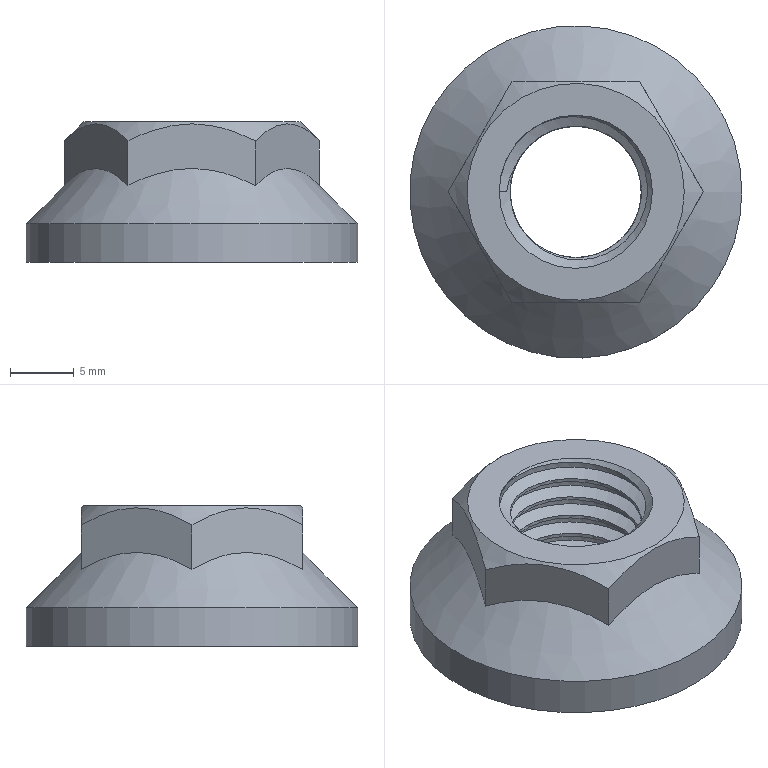Part | NX | features CYLINDER 2, DATUM_CSYS 2, CHAMFER 1, CONE 1, DELETE FACE 1, EXTRUDE 1, HOLE PACKAGE 1, INTERSECT 1, SIMPLE HOLE 1, SKETCH 1, SYMBOLIC_THREAD 1, THREADS 1 | 1 solid | 19 faces | box 26 x 26 x 11 mm | volume 3067 mm3 | plane 10 | cone 4 | cylinder 3 | spline 2 | commonest cylinder face diameters 10.3 x1 12 x1 26 x1
STEP:
#1=CARTESIAN_POINT('',(-4.994,-8.65,9.5));
#2=VERTEX_POINT('',#1);
#3=CARTESIAN_POINT('',(-4.994,-8.65,6.012));
#4=VERTEX_POINT('',#3);
#5=CARTESIAN_POINT('',(-4.994,-8.65,11.));
#6=DIRECTION('',(0.,0.,-1.));
#7=VECTOR('',#6,1000.);
#8=LINE('',#5,#7);
#9=EDGE_CURVE('',#2,#4,#8,.T.);
#10=ORIENTED_EDGE('',*,*,#9,.T.);
#11=CARTESIAN_POINT('',(4.994,-8.65,6.012));
#12=VERTEX_POINT('',#11);
#13=CARTESIAN_POINT('',(-4.994,-8.65,6.012));
#14=CARTESIAN_POINT('',(-3.437,-8.65,6.79));
#15=CARTESIAN_POINT('',(0.004869,-8.65,7.912));
#16=CARTESIAN_POINT('',(3.447,-8.65,6.785));
#17=CARTESIAN_POINT('',(4.994,-8.65,6.012));
#18=B_SPLINE_CURVE_WITH_KNOTS('',3,(#13,#14,#15,#16,#17),.UNSPECIFIED.,.F.,.F.,(4,1,4),(0.008324,0.01351,0.01869),.UNSPECIFIED.);
#19=EDGE_CURVE('',#4,#12,#18,.T.);
#20=ORIENTED_EDGE('',*,*,#19,.T.);
#21=CARTESIAN_POINT('',(4.994,-8.65,9.5));
#22=VERTEX_POINT('',#21);
#23=CARTESIAN_POINT('',(4.994,-8.65,11.));
#24=DIRECTION('',(0.,0.,-1.));
#25=VECTOR('',#24,1000.);
#26=LINE('',#23,#25);
#27=EDGE_CURVE('',#22,#12,#26,.T.);
#28=ORIENTED_EDGE('',*,*,#27,.F.);
#29=CARTESIAN_POINT('',(-4.994,-8.65,9.5));
#30=CARTESIAN_POINT('',(-3.445,-8.65,10.275));
#31=CARTESIAN_POINT('',(0.002531,-8.65,11.403));
#32=CARTESIAN_POINT('',(3.449,-8.65,10.273));
#33=CARTESIAN_POINT('',(4.994,-8.65,9.5));
#34=B_SPLINE_CURVE_WITH_KNOTS('',3,(#29,#30,#31,#32,#33),.UNSPECIFIED.,.F.,.F.,(4,1,4),(0.006405,0.01158,0.01676),.UNSPECIFIED.);
#35=EDGE_CURVE('',#22,#2,#34,.F.);
#36=ORIENTED_EDGE('',*,*,#35,.T.);
#37=EDGE_LOOP('',(#10,#20,#28,#36));
#38=FACE_BOUND('',#37,.T.);
#39=CARTESIAN_POINT('',(-4.994,-8.65,11.));
#40=DIRECTION('',(0.,1.,0.));
#41=DIRECTION('',(-1.,0.,0.));
#42=AXIS2_PLACEMENT_3D('',#39,#40,#41);
#43=PLANE('',#42);
#44=ADVANCED_FACE('',(#38),#43,.F.);
#45=ORIENTED_EDGE('',*,*,#27,.T.);
#46=CARTESIAN_POINT('',(9.988,0.,6.012));
#47=VERTEX_POINT('',#46);
#48=CARTESIAN_POINT('',(4.994,-8.65,6.012));
#49=CARTESIAN_POINT('',(5.384,-7.974,6.402));
#50=CARTESIAN_POINT('',(6.177,-6.602,7.066));
#51=CARTESIAN_POINT('',(7.921,-3.581,7.631));
#52=CARTESIAN_POINT('',(9.203,-1.36,6.797));
#53=CARTESIAN_POINT('',(9.988,0.,6.012));
#54=B_SPLINE_CURVE_WITH_KNOTS('',3,(#48,#49,#50,#51,#52,#53),.UNSPECIFIED.,.F.,.F.,(4,1,1,4),(0.000000254,0.00258,0.005159,0.01032),.UNSPECIFIED.);
#55=EDGE_CURVE('',#12,#47,#54,.T.);
#56=ORIENTED_EDGE('',*,*,#55,.T.);
#57=CARTESIAN_POINT('',(9.988,0.,9.5));
#58=VERTEX_POINT('',#57);
#59=CARTESIAN_POINT('',(9.988,0.,11.));
#60=DIRECTION('',(0.,0.,-1.));
#61=VECTOR('',#60,1000.);
#62=LINE('',#59,#61);
#63=EDGE_CURVE('',#58,#47,#62,.T.);
#64=ORIENTED_EDGE('',*,*,#63,.F.);
#65=CARTESIAN_POINT('',(9.988,0.,9.5));
#66=CARTESIAN_POINT('',(9.598,-0.6758,9.89));
#67=CARTESIAN_POINT('',(8.806,-2.048,10.554));
#68=CARTESIAN_POINT('',(7.061,-5.069,11.119));
#69=CARTESIAN_POINT('',(5.779,-7.29,10.285));
#70=CARTESIAN_POINT('',(4.994,-8.65,9.5));
#71=B_SPLINE_CURVE_WITH_KNOTS('',3,(#65,#66,#67,#68,#69,#70),.UNSPECIFIED.,.F.,.F.,(4,1,1,4),(0.000000254,0.00258,0.005159,0.01032),.UNSPECIFIED.);
#72=EDGE_CURVE('',#58,#22,#71,.T.);
#73=ORIENTED_EDGE('',*,*,#72,.T.);
#74=EDGE_LOOP('',(#45,#56,#64,#73));
#75=FACE_BOUND('',#74,.T.);
#76=CARTESIAN_POINT('',(4.994,-8.65,11.));
#77=DIRECTION('',(-0.866,0.5,0.));
#78=DIRECTION('',(-0.5,-0.866,0.));
#79=AXIS2_PLACEMENT_3D('',#76,#77,#78);
#80=PLANE('',#79);
#81=ADVANCED_FACE('',(#75),#80,.F.);
#82=ORIENTED_EDGE('',*,*,#63,.T.);
#83=CARTESIAN_POINT('',(4.994,8.65,6.012));
#84=VERTEX_POINT('',#83);
#85=CARTESIAN_POINT('',(9.988,0.,6.012));
#86=CARTESIAN_POINT('',(9.598,0.6758,6.402));
#87=CARTESIAN_POINT('',(8.806,2.048,7.066));
#88=CARTESIAN_POINT('',(7.061,5.069,7.631));
#89=CARTESIAN_POINT('',(5.779,7.29,6.797));
#90=CARTESIAN_POINT('',(4.994,8.65,6.012));
#91=B_SPLINE_CURVE_WITH_KNOTS('',3,(#85,#86,#87,#88,#89,#90),.UNSPECIFIED.,.F.,.F.,(4,1,1,4),(0.000000254,0.00258,0.005159,0.01032),.UNSPECIFIED.);
#92=EDGE_CURVE('',#47,#84,#91,.T.);
#93=ORIENTED_EDGE('',*,*,#92,.T.);
#94=CARTESIAN_POINT('',(4.994,8.65,9.5));
#95=VERTEX_POINT('',#94);
#96=CARTESIAN_POINT('',(4.994,8.65,11.));
#97=DIRECTION('',(0.,0.,-1.));
#98=VECTOR('',#97,1000.);
#99=LINE('',#96,#98);
#100=EDGE_CURVE('',#95,#84,#99,.T.);
#101=ORIENTED_EDGE('',*,*,#100,.F.);
#102=CARTESIAN_POINT('',(4.994,8.65,9.5));
#103=CARTESIAN_POINT('',(5.384,7.974,9.89));
#104=CARTESIAN_POINT('',(6.177,6.602,10.554));
#105=CARTESIAN_POINT('',(7.921,3.581,11.119));
#106=CARTESIAN_POINT('',(9.203,1.36,10.285));
#107=CARTESIAN_POINT('',(9.988,0.,9.5));
#108=B_SPLINE_CURVE_WITH_KNOTS('',3,(#102,#103,#104,#105,#106,#107),.UNSPECIFIED.,.F.,.F.,(4,1,1,4),(0.000000254,0.00258,0.005159,0.01032),.UNSPECIFIED.);
#109=EDGE_CURVE('',#95,#58,#108,.T.);
#110=ORIENTED_EDGE('',*,*,#109,.T.);
#111=EDGE_LOOP('',(#82,#93,#101,#110));
#112=FACE_BOUND('',#111,.T.);
#113=CARTESIAN_POINT('',(9.988,0.,11.));
#114=DIRECTION('',(-0.866,-0.5,0.));
#115=DIRECTION('',(0.5,-0.866,0.));
#116=AXIS2_PLACEMENT_3D('',#113,#114,#115);
#117=PLANE('',#116);
#118=ADVANCED_FACE('',(#112),#117,.F.);
#119=ORIENTED_EDGE('',*,*,#100,.T.);
#120=CARTESIAN_POINT('',(-4.994,8.65,6.012));
#121=VERTEX_POINT('',#120);
#122=CARTESIAN_POINT('',(-4.994,8.65,6.012));
#123=CARTESIAN_POINT('',(-3.437,8.65,6.79));
#124=CARTESIAN_POINT('',(0.004869,8.65,7.912));
#125=CARTESIAN_POINT('',(3.447,8.65,6.785));
#126=CARTESIAN_POINT('',(4.994,8.65,6.012));
#127=B_SPLINE_CURVE_WITH_KNOTS('',3,(#122,#123,#124,#125,#126),.UNSPECIFIED.,.F.,.F.,(4,1,4),(0.008324,0.01351,0.01869),.UNSPECIFIED.);
#128=EDGE_CURVE('',#84,#121,#127,.F.);
#129=ORIENTED_EDGE('',*,*,#128,.T.);
#130=CARTESIAN_POINT('',(-4.994,8.65,9.5));
#131=VERTEX_POINT('',#130);
#132=CARTESIAN_POINT('',(-4.994,8.65,11.));
#133=DIRECTION('',(0.,0.,-1.));
#134=VECTOR('',#133,1000.);
#135=LINE('',#132,#134);
#136=EDGE_CURVE('',#131,#121,#135,.T.);
#137=ORIENTED_EDGE('',*,*,#136,.F.);
#138=CARTESIAN_POINT('',(-4.994,8.65,9.5));
#139=CARTESIAN_POINT('',(-3.445,8.65,10.275));
#140=CARTESIAN_POINT('',(0.002531,8.65,11.403));
#141=CARTESIAN_POINT('',(3.449,8.65,10.273));
#142=CARTESIAN_POINT('',(4.994,8.65,9.5));
#143=B_SPLINE_CURVE_WITH_KNOTS('',3,(#138,#139,#140,#141,#142),.UNSPECIFIED.,.F.,.F.,(4,1,4),(0.006405,0.01158,0.01676),.UNSPECIFIED.);
#144=EDGE_CURVE('',#131,#95,#143,.T.);
#145=ORIENTED_EDGE('',*,*,#144,.T.);
#146=EDGE_LOOP('',(#119,#129,#137,#145));
#147=FACE_BOUND('',#146,.T.);
#148=CARTESIAN_POINT('',(4.994,8.65,11.));
#149=DIRECTION('',(0.,-1.,0.));
#150=DIRECTION('',(1.,0.,0.));
#151=AXIS2_PLACEMENT_3D('',#148,#149,#150);
#152=PLANE('',#151);
#153=ADVANCED_FACE('',(#147),#152,.F.);
#154=ORIENTED_EDGE('',*,*,#136,.T.);
#155=CARTESIAN_POINT('',(-9.988,0.,6.012));
#156=VERTEX_POINT('',#155);
#157=CARTESIAN_POINT('',(-4.994,8.65,6.012));
#158=CARTESIAN_POINT('',(-5.384,7.974,6.402));
#159=CARTESIAN_POINT('',(-6.177,6.602,7.066));
#160=CARTESIAN_POINT('',(-7.921,3.581,7.631));
#161=CARTESIAN_POINT('',(-9.203,1.36,6.797));
#162=CARTESIAN_POINT('',(-9.988,0.,6.012));
#163=B_SPLINE_CURVE_WITH_KNOTS('',3,(#157,#158,#159,#160,#161,#162),.UNSPECIFIED.,.F.,.F.,(4,1,1,4),(0.000000254,0.00258,0.005159,0.01032),.UNSPECIFIED.);
#164=EDGE_CURVE('',#121,#156,#163,.T.);
#165=ORIENTED_EDGE('',*,*,#164,.T.);
#166=CARTESIAN_POINT('',(-9.988,0.,9.5));
#167=VERTEX_POINT('',#166);
#168=CARTESIAN_POINT('',(-9.988,0.,11.));
#169=DIRECTION('',(0.,0.,-1.));
#170=VECTOR('',#169,1000.);
#171=LINE('',#168,#170);
#172=EDGE_CURVE('',#167,#156,#171,.T.);
#173=ORIENTED_EDGE('',*,*,#172,.F.);
#174=CARTESIAN_POINT('',(-9.988,0.,9.5));
#175=CARTESIAN_POINT('',(-9.598,0.6758,9.89));
#176=CARTESIAN_POINT('',(-8.806,2.048,10.554));
#177=CARTESIAN_POINT('',(-7.061,5.069,11.119));
#178=CARTESIAN_POINT('',(-5.779,7.29,10.285));
#179=CARTESIAN_POINT('',(-4.994,8.65,9.5));
#180=B_SPLINE_CURVE_WITH_KNOTS('',3,(#174,#175,#176,#177,#178,#179),.UNSPECIFIED.,.F.,.F.,(4,1,1,4),(0.000000254,0.00258,0.005159,0.01032),.UNSPECIFIED.);
#181=EDGE_CURVE('',#167,#131,#180,.T.);
#182=ORIENTED_EDGE('',*,*,#181,.T.);
#183=EDGE_LOOP('',(#154,#165,#173,#182));
#184=FACE_BOUND('',#183,.T.);
#185=CARTESIAN_POINT('',(-4.994,8.65,11.));
#186=DIRECTION('',(0.866,-0.5,0.));
#187=DIRECTION('',(0.5,0.866,0.));
#188=AXIS2_PLACEMENT_3D('',#185,#186,#187);
#189=PLANE('',#188);
#190=ADVANCED_FACE('',(#184),#189,.F.);
#191=ORIENTED_EDGE('',*,*,#172,.T.);
#192=CARTESIAN_POINT('',(-9.988,0.,6.012));
#193=CARTESIAN_POINT('',(-9.598,-0.6758,6.402));
#194=CARTESIAN_POINT('',(-8.806,-2.048,7.066));
#195=CARTESIAN_POINT('',(-7.061,-5.069,7.631));
#196=CARTESIAN_POINT('',(-5.779,-7.29,6.797));
#197=CARTESIAN_POINT('',(-4.994,-8.65,6.012));
#198=B_SPLINE_CURVE_WITH_KNOTS('',3,(#192,#193,#194,#195,#196,#197),.UNSPECIFIED.,.F.,.F.,(4,1,1,4),(0.000000254,0.00258,0.005159,0.01032),.UNSPECIFIED.);
#199=EDGE_CURVE('',#156,#4,#198,.T.);
#200=ORIENTED_EDGE('',*,*,#199,.T.);
#201=ORIENTED_EDGE('',*,*,#9,.F.);
#202=CARTESIAN_POINT('',(-4.994,-8.65,9.5));
#203=CARTESIAN_POINT('',(-5.384,-7.974,9.89));
#204=CARTESIAN_POINT('',(-6.177,-6.602,10.554));
#205=CARTESIAN_POINT('',(-7.921,-3.581,11.119));
#206=CARTESIAN_POINT('',(-9.203,-1.36,10.285));
#207=CARTESIAN_POINT('',(-9.988,0.,9.5));
#208=B_SPLINE_CURVE_WITH_KNOTS('',3,(#202,#203,#204,#205,#206,#207),.UNSPECIFIED.,.F.,.F.,(4,1,1,4),(0.000000254,0.00258,0.005159,0.01032),.UNSPECIFIED.);
#209=EDGE_CURVE('',#2,#167,#208,.T.);
#210=ORIENTED_EDGE('',*,*,#209,.T.);
#211=EDGE_LOOP('',(#191,#200,#201,#210));
#212=FACE_BOUND('',#211,.T.);
#213=CARTESIAN_POINT('',(-9.988,0.,11.));
#214=DIRECTION('',(0.866,0.5,0.));
#215=DIRECTION('',(-0.5,0.866,0.));
#216=AXIS2_PLACEMENT_3D('',#213,#214,#215);
#217=PLANE('',#216);
#218=ADVANCED_FACE('',(#212),#217,.F.);
#219=CARTESIAN_POINT('',(-6.,0.,11.));
#220=VERTEX_POINT('',#219);
#221=CARTESIAN_POINT('',(-3.737,4.694,11.));
#222=VERTEX_POINT('',#221);
#223=CARTESIAN_POINT('',(0.,0.,11.));
#224=DIRECTION('',(0.,0.,1.));
#225=DIRECTION('',(1.,0.,0.));
#226=AXIS2_PLACEMENT_3D('',#223,#224,#225);
#227=CIRCLE('',#226,6.);
#228=EDGE_CURVE('',#220,#222,#227,.F.);
#229=ORIENTED_EDGE('',*,*,#228,.T.);
#230=CARTESIAN_POINT('',(0.,0.,11.));
#231=DIRECTION('',(0.,0.,1.));
#232=DIRECTION('',(1.,0.,0.));
#233=AXIS2_PLACEMENT_3D('',#230,#231,#232);
#234=CIRCLE('',#233,6.);
#235=EDGE_CURVE('',#222,#220,#234,.F.);
#236=ORIENTED_EDGE('',*,*,#235,.T.);
#237=EDGE_LOOP('',(#229,#236));
#238=FACE_BOUND('',#237,.T.);
#239=CARTESIAN_POINT('',(8.488,0.,11.));
#240=VERTEX_POINT('',#239);
#241=CARTESIAN_POINT('',(0.,0.,11.));
#242=DIRECTION('',(0.,0.,1.));
#243=DIRECTION('',(1.,0.,0.));
#244=AXIS2_PLACEMENT_3D('',#241,#242,#243);
#245=CIRCLE('',#244,8.488);
#246=EDGE_CURVE('',#240,#240,#245,.T.);
#247=ORIENTED_EDGE('',*,*,#246,.T.);
#248=EDGE_LOOP('',(#247));
#249=FACE_BOUND('',#248,.T.);
#250=CARTESIAN_POINT('',(0.,0.,11.));
#251=DIRECTION('',(0.,0.,1.));
#252=DIRECTION('',(1.,0.,0.));
#253=AXIS2_PLACEMENT_3D('',#250,#251,#252);
#254=PLANE('',#253);
#255=ADVANCED_FACE('',(#238,#249),#254,.T.);
#256=ORIENTED_EDGE('',*,*,#246,.F.);
#257=EDGE_LOOP('',(#256));
#258=FACE_BOUND('',#257,.T.);
#259=ORIENTED_EDGE('',*,*,#35,.F.);
#260=ORIENTED_EDGE('',*,*,#72,.F.);
#261=ORIENTED_EDGE('',*,*,#109,.F.);
#262=ORIENTED_EDGE('',*,*,#144,.F.);
#263=ORIENTED_EDGE('',*,*,#181,.F.);
#264=ORIENTED_EDGE('',*,*,#209,.F.);
#265=EDGE_LOOP('',(#259,#260,#261,#262,#263,#264));
#266=FACE_BOUND('',#265,.T.);
#267=CARTESIAN_POINT('',(0.,0.,9.5));
#268=DIRECTION('',(0.,0.,-1.));
#269=DIRECTION('',(-1.,0.,0.));
#270=AXIS2_PLACEMENT_3D('',#267,#268,#269);
#271=CONICAL_SURFACE('',#270,9.988,0.7854);
#272=ADVANCED_FACE('',(#258,#266),#271,.T.);
#273=CARTESIAN_POINT('',(13.,0.,3.));
#274=VERTEX_POINT('',#273);
#275=CARTESIAN_POINT('',(0.,0.,3.));
#276=DIRECTION('',(0.,0.,1.));
#277=DIRECTION('',(1.,0.,0.));
#278=AXIS2_PLACEMENT_3D('',#275,#276,#277);
#279=CIRCLE('',#278,13.);
#280=EDGE_CURVE('',#274,#274,#279,.T.);
#281=ORIENTED_EDGE('',*,*,#280,.T.);
#282=EDGE_LOOP('',(#281));
#283=FACE_BOUND('',#282,.T.);
#284=ORIENTED_EDGE('',*,*,#19,.F.);
#285=ORIENTED_EDGE('',*,*,#199,.F.);
#286=ORIENTED_EDGE('',*,*,#164,.F.);
#287=ORIENTED_EDGE('',*,*,#128,.F.);
#288=ORIENTED_EDGE('',*,*,#92,.F.);
#289=ORIENTED_EDGE('',*,*,#55,.F.);
#290=EDGE_LOOP('',(#284,#285,#286,#287,#288,#289));
#291=FACE_BOUND('',#290,.T.);
#292=CARTESIAN_POINT('',(0.,0.,16.));
#293=DIRECTION('',(0.,0.,-1.));
#294=DIRECTION('',(1.,0.,0.));
#295=AXIS2_PLACEMENT_3D('',#292,#293,#294);
#296=CONICAL_SURFACE('',#295,0.,0.7854);
#297=ADVANCED_FACE('',(#283,#291),#296,.T.);
#298=CARTESIAN_POINT('',(-6.,0.,0.));
#299=VERTEX_POINT('',#298);
#300=CARTESIAN_POINT('',(0.,0.,0.));
#301=DIRECTION('',(0.,0.,-1.));
#302=DIRECTION('',(-1.,0.,0.));
#303=AXIS2_PLACEMENT_3D('',#300,#301,#302);
#304=CIRCLE('',#303,6.);
#305=EDGE_CURVE('',#299,#299,#304,.F.);
#306=ORIENTED_EDGE('',*,*,#305,.T.);
#307=EDGE_LOOP('',(#306));
#308=FACE_BOUND('',#307,.T.);
#309=CARTESIAN_POINT('',(13.,0.,0.));
#310=VERTEX_POINT('',#309);
#311=CARTESIAN_POINT('',(0.,0.,0.));
#312=DIRECTION('',(0.,0.,1.));
#313=DIRECTION('',(1.,0.,0.));
#314=AXIS2_PLACEMENT_3D('',#311,#312,#313);
#315=CIRCLE('',#314,13.);
#316=EDGE_CURVE('',#310,#310,#315,.T.);
#317=ORIENTED_EDGE('',*,*,#316,.F.);
#318=EDGE_LOOP('',(#317));
#319=FACE_BOUND('',#318,.T.);
#320=CARTESIAN_POINT('',(0.,0.,0.));
#321=DIRECTION('',(0.,0.,-1.));
#322=DIRECTION('',(-1.,0.,0.));
#323=AXIS2_PLACEMENT_3D('',#320,#321,#322);
#324=PLANE('',#323);
#325=ADVANCED_FACE('',(#308,#319),#324,.T.);
#326=ORIENTED_EDGE('',*,*,#280,.F.);
#327=EDGE_LOOP('',(#326));
#328=FACE_BOUND('',#327,.T.);
#329=ORIENTED_EDGE('',*,*,#316,.T.);
#330=EDGE_LOOP('',(#329));
#331=FACE_BOUND('',#330,.T.);
#332=CARTESIAN_POINT('',(0.,0.,0.));
#333=DIRECTION('',(0.,0.,1.));
#334=DIRECTION('',(1.,0.,0.));
#335=AXIS2_PLACEMENT_3D('',#332,#333,#334);
#336=CYLINDRICAL_SURFACE('',#335,13.);
#337=ADVANCED_FACE('',(#328,#331),#336,.T.);
#338=CARTESIAN_POINT('',(-4.333,-2.784,10.15));
#339=VERTEX_POINT('',#338);
#340=CARTESIAN_POINT('',(4.339,2.774,2.274));
#341=VERTEX_POINT('',#340);
#342=CARTESIAN_POINT('',(-4.333,-2.784,10.15));
#343=CARTESIAN_POINT('',(-5.161,-1.496,10.067));
#344=CARTESIAN_POINT('',(-5.577,1.793,9.904));
#345=CARTESIAN_POINT('',(-2.144,5.461,9.658));
#346=CARTESIAN_POINT('',(2.855,5.122,9.412));
#347=CARTESIAN_POINT('',(5.773,1.04,9.166));
#348=CARTESIAN_POINT('',(4.463,-3.803,8.919));
#349=CARTESIAN_POINT('',(-0.1032,-5.864,8.674));
#350=CARTESIAN_POINT('',(-4.603,-3.635,8.427));
#351=CARTESIAN_POINT('',(-5.73,1.246,8.181));
#352=CARTESIAN_POINT('',(-2.671,5.223,7.935));
#353=CARTESIAN_POINT('',(2.346,5.375,7.689));
#354=CARTESIAN_POINT('',(5.641,1.603,7.443));
#355=CARTESIAN_POINT('',(4.815,-3.349,7.197));
#356=CARTESIAN_POINT('',(0.4676,-5.845,6.951));
#357=CARTESIAN_POINT('',(-4.222,-4.072,6.705));
#358=CARTESIAN_POINT('',(-5.824,0.6857,6.458));
#359=CARTESIAN_POINT('',(-3.17,4.933,6.213));
#360=CARTESIAN_POINT('',(1.807,5.581,5.966));
#361=CARTESIAN_POINT('',(5.459,2.141,5.72));
#362=CARTESIAN_POINT('',(5.122,-2.858,5.474));
#363=CARTESIAN_POINT('',(1.034,-5.773,5.228));
#364=CARTESIAN_POINT('',(-3.802,-4.464,4.982));
#365=CARTESIAN_POINT('',(-5.865,0.1088,4.736));
#366=CARTESIAN_POINT('',(-3.632,4.604,4.489));
#367=CARTESIAN_POINT('',(1.248,5.73,4.244));
#368=CARTESIAN_POINT('',(5.225,2.666,3.997));
#369=CARTESIAN_POINT('',(5.374,-2.345,3.752));
#370=CARTESIAN_POINT('',(1.599,-5.644,3.505));
#371=CARTESIAN_POINT('',(-3.352,-4.812,3.259));
#372=CARTESIAN_POINT('',(-5.845,-0.4681,3.013));
#373=CARTESIAN_POINT('',(-4.069,4.228,2.767));
#374=CARTESIAN_POINT('',(0.6899,5.818,2.521));
#375=CARTESIAN_POINT('',(3.514,4.065,2.357));
#376=CARTESIAN_POINT('',(4.339,2.774,2.274));
#377=B_SPLINE_CURVE_WITH_KNOTS('',3,(#342,#343,#344,#345,#346,#347,#348,#349,#350,#351,#352,#353,#354,#355,#356,#357,#358,#359,#360,#361,#362,#363,#364,#365,#366,#367,#368,#369,#370,#371,#372,#373,#374,#375,#376),.UNSPECIFIED.,.F.,.F.,(4,1,1,1,1,1,1,1,1,1,1,1,1,1,1,1,1,1,1,1,1,1,1,1,1,1,1,1,1,1,1,1,4),(0.,0.004536,0.009071,0.01361,0.01814,0.02268,0.02721,0.03175,0.03629,0.04082,0.04536,0.04989,0.05443,0.05896,0.0635,0.06803,0.07257,0.07711,0.08164,0.08618,0.09071,0.09525,0.09978,0.1043,0.1089,0.1134,0.1179,0.1225,0.127,0.1315,0.1361,0.1406,0.1451),.UNSPECIFIED.);
#378=EDGE_CURVE('',#339,#341,#377,.T.);
#379=ORIENTED_EDGE('',*,*,#378,.T.);
#380=CARTESIAN_POINT('',(4.339,2.774,0.85));
#381=VERTEX_POINT('',#380);
#382=CARTESIAN_POINT('',(4.339,2.774,11.));
#383=DIRECTION('',(0.,0.,-1.));
#384=VECTOR('',#383,1000.);
#385=LINE('',#382,#384);
#386=EDGE_CURVE('',#341,#381,#385,.T.);
#387=ORIENTED_EDGE('',*,*,#386,.T.);
#388=CARTESIAN_POINT('',(3.676,3.607,0.85));
#389=VERTEX_POINT('',#388);
#390=CARTESIAN_POINT('',(0.,0.,0.85));
#391=DIRECTION('',(0.,0.,-1.));
#392=DIRECTION('',(-1.,0.,0.));
#393=AXIS2_PLACEMENT_3D('',#390,#391,#392);
#394=CIRCLE('',#393,5.15);
#395=EDGE_CURVE('',#381,#389,#394,.T.);
#396=ORIENTED_EDGE('',*,*,#395,.T.);
#397=CARTESIAN_POINT('',(-4.761,1.962,10.15));
#398=VERTEX_POINT('',#397);
#399=CARTESIAN_POINT('',(3.676,3.607,0.85));
#400=CARTESIAN_POINT('',(2.409,4.898,0.9477));
#401=CARTESIAN_POINT('',(-1.51,5.972,1.141));
#402=CARTESIAN_POINT('',(-5.937,1.699,1.432));
#403=CARTESIAN_POINT('',(-4.452,-4.275,1.722));
#404=CARTESIAN_POINT('',(1.452,-5.998,2.013));
#405=CARTESIAN_POINT('',(5.914,-1.765,2.303));
#406=CARTESIAN_POINT('',(4.502,4.222,2.594));
#407=CARTESIAN_POINT('',(-1.382,6.015,2.885));
#408=CARTESIAN_POINT('',(-5.893,1.834,3.175));
#409=CARTESIAN_POINT('',(-4.551,-4.17,3.465));
#410=CARTESIAN_POINT('',(1.313,-6.031,3.756));
#411=CARTESIAN_POINT('',(5.873,-1.899,4.047));
#412=CARTESIAN_POINT('',(4.596,4.121,4.337));
#413=CARTESIAN_POINT('',(-1.249,6.044,4.628));
#414=CARTESIAN_POINT('',(-5.851,1.963,4.919));
#415=CARTESIAN_POINT('',(-4.641,-4.068,5.209));
#416=CARTESIAN_POINT('',(1.179,-6.058,5.5));
#417=CARTESIAN_POINT('',(5.828,-2.031,5.791));
#418=CARTESIAN_POINT('',(4.688,4.014,6.081));
#419=CARTESIAN_POINT('',(-1.108,6.071,6.372));
#420=CARTESIAN_POINT('',(-5.804,2.098,6.662));
#421=CARTESIAN_POINT('',(-4.734,-3.96,6.953));
#422=CARTESIAN_POINT('',(1.04,-6.084,7.244));
#423=CARTESIAN_POINT('',(5.782,-2.161,7.534));
#424=CARTESIAN_POINT('',(4.777,3.909,7.825));
#425=CARTESIAN_POINT('',(-0.9743,6.095,8.116));
#426=CARTESIAN_POINT('',(-5.757,2.225,8.406));
#427=CARTESIAN_POINT('',(-4.82,-3.854,8.697));
#428=CARTESIAN_POINT('',(0.9037,-6.105,8.988));
#429=CARTESIAN_POINT('',(5.73,-2.293,9.278));
#430=CARTESIAN_POINT('',(4.866,3.8,9.569));
#431=CARTESIAN_POINT('',(-0.8359,6.105,9.86));
#432=CARTESIAN_POINT('',(-4.072,3.634,10.052));
#433=CARTESIAN_POINT('',(-4.761,1.962,10.15));
#434=B_SPLINE_CURVE_WITH_KNOTS('',3,(#399,#400,#401,#402,#403,#404,#405,#406,#407,#408,#409,#410,#411,#412,#413,#414,#415,#416,#417,#418,#419,#420,#421,#422,#423,#424,#425,#426,#427,#428,#429,#430,#431,#432,#433),.UNSPECIFIED.,.F.,.F.,(4,1,1,1,1,1,1,1,1,1,1,1,1,1,1,1,1,1,1,1,1,1,1,1,1,1,1,1,1,1,1,1,4),(0.,0.005356,0.01071,0.01607,0.02142,0.02678,0.03214,0.03749,0.04285,0.0482,0.05356,0.05892,0.06427,0.06963,0.07498,0.08034,0.0857,0.09105,0.09641,0.1018,0.1071,0.1125,0.1178,0.1232,0.1285,0.1339,0.1393,0.1446,0.15,0.1553,0.1607,0.166,0.1714),.UNSPECIFIED.);
#435=EDGE_CURVE('',#389,#398,#434,.T.);
#436=ORIENTED_EDGE('',*,*,#435,.T.);
#437=CARTESIAN_POINT('',(0.,0.,10.15));
#438=DIRECTION('',(0.,0.,1.));
#439=DIRECTION('',(1.,0.,0.));
#440=AXIS2_PLACEMENT_3D('',#437,#438,#439);
#441=CIRCLE('',#440,5.15);
#442=EDGE_CURVE('',#398,#339,#441,.T.);
#443=ORIENTED_EDGE('',*,*,#442,.T.);
#444=EDGE_LOOP('',(#379,#387,#396,#436,#443));
#445=FACE_BOUND('',#444,.T.);
#446=CARTESIAN_POINT('',(0.,0.,11.));
#447=DIRECTION('',(0.,0.,-1.));
#448=DIRECTION('',(-1.,0.,0.));
#449=AXIS2_PLACEMENT_3D('',#446,#447,#448);
#450=CYLINDRICAL_SURFACE('',#449,5.15);
#451=ADVANCED_FACE('',(#445),#450,.F.);
#452=CARTESIAN_POINT('',(-4.333,-2.784,10.15));
#453=CARTESIAN_POINT('',(-3.755,-3.755,10.189));
#454=CARTESIAN_POINT('',(-1.974,-5.272,10.264));
#455=CARTESIAN_POINT('',(1.549,-5.524,10.376));
#456=CARTESIAN_POINT('',(4.54,-3.668,10.485));
#457=CARTESIAN_POINT('',(5.922,-0.4368,10.592));
#458=CARTESIAN_POINT('',(5.234,3.004,10.696));
#459=CARTESIAN_POINT('',(2.758,5.476,10.799));
#460=CARTESIAN_POINT('',(-0.6604,6.19,10.901));
#461=CARTESIAN_POINT('',(-2.834,5.37,10.967));
#462=CARTESIAN_POINT('',(-3.737,4.694,11.));
#463=B_SPLINE_CURVE_WITH_KNOTS('',3,(#452,#453,#454,#455,#456,#457,#458,#459,#460,#461,#462),.UNSPECIFIED.,.F.,.F.,(4,1,1,1,1,1,1,1,4),(0.,0.003343,0.006686,0.01003,0.01337,0.01671,0.02006,0.0234,0.02674),.UNSPECIFIED.);
#464=EDGE_CURVE('',#339,#222,#463,.T.);
#465=ORIENTED_EDGE('',*,*,#464,.F.);
#466=ORIENTED_EDGE('',*,*,#442,.F.);
#467=CARTESIAN_POINT('',(-5.408,0.,10.408));
#468=VERTEX_POINT('',#467);
#469=CARTESIAN_POINT('',(-5.408,0.,10.408));
#470=CARTESIAN_POINT('',(-5.323,0.694,10.323));
#471=CARTESIAN_POINT('',(-5.108,1.355,10.239));
#472=CARTESIAN_POINT('',(-4.761,1.962,10.15));
#473=B_SPLINE_CURVE_WITH_KNOTS('',3,(#469,#470,#471,#472),.UNSPECIFIED.,.F.,.F.,(4,4),(0.,0.002083),.UNSPECIFIED.);
#474=EDGE_CURVE('',#468,#398,#473,.T.);
#475=ORIENTED_EDGE('',*,*,#474,.F.);
#476=CARTESIAN_POINT('',(0.,0.,5.));
#477=DIRECTION('',(0.7071,0.,-0.7071));
#478=VECTOR('',#477,1000.);
#479=LINE('',#476,#478);
#480=EDGE_CURVE('',#220,#468,#479,.T.);
#481=ORIENTED_EDGE('',*,*,#480,.F.);
#482=ORIENTED_EDGE('',*,*,#235,.F.);
#483=EDGE_LOOP('',(#465,#466,#475,#481,#482));
#484=FACE_BOUND('',#483,.T.);
#485=CARTESIAN_POINT('',(0.,0.,11.));
#486=DIRECTION('',(0.,0.,1.));
#487=DIRECTION('',(1.,0.,0.));
#488=AXIS2_PLACEMENT_3D('',#485,#486,#487);
#489=CONICAL_SURFACE('',#488,6.,0.7854);
#490=ADVANCED_FACE('',(#484),#489,.F.);
#491=CARTESIAN_POINT('',(4.37,2.794,0.8136));
#492=VERTEX_POINT('',#491);
#493=CARTESIAN_POINT('',(0.,0.,6.));
#494=DIRECTION('',(-0.5957,-0.3809,0.7071));
#495=VECTOR('',#494,1000.);
#496=LINE('',#493,#495);
#497=EDGE_CURVE('',#492,#381,#496,.T.);
#498=ORIENTED_EDGE('',*,*,#497,.F.);
#499=CARTESIAN_POINT('',(3.676,3.607,0.85));
#500=CARTESIAN_POINT('',(3.935,3.36,0.8377));
#501=CARTESIAN_POINT('',(4.166,3.089,0.8258));
#502=CARTESIAN_POINT('',(4.37,2.794,0.8136));
#503=B_SPLINE_CURVE_WITH_KNOTS('',3,(#499,#500,#501,#502),.UNSPECIFIED.,.F.,.F.,(4,4),(0.,0.00107),.UNSPECIFIED.);
#504=EDGE_CURVE('',#389,#492,#503,.T.);
#505=ORIENTED_EDGE('',*,*,#504,.F.);
#506=ORIENTED_EDGE('',*,*,#395,.F.);
#507=EDGE_LOOP('',(#498,#505,#506));
#508=FACE_BOUND('',#507,.T.);
#509=ORIENTED_EDGE('',*,*,#305,.F.);
#510=EDGE_LOOP('',(#509));
#511=FACE_BOUND('',#510,.T.);
#512=CARTESIAN_POINT('',(0.,0.,0.85));
#513=DIRECTION('',(0.,0.,-1.));
#514=DIRECTION('',(-1.,0.,0.));
#515=AXIS2_PLACEMENT_3D('',#512,#513,#514);
#516=CONICAL_SURFACE('',#515,5.15,0.7854);
#517=ADVANCED_FACE('',(#508,#511),#516,.F.);
#518=CARTESIAN_POINT('',(5.055,3.232,1.784));
#519=VERTEX_POINT('',#518);
#520=CARTESIAN_POINT('',(5.307,3.393,1.611));
#521=CARTESIAN_POINT('',(4.33,2.769,2.28));
#522=B_SPLINE_CURVE_WITH_KNOTS('',1,(#520,#521),.UNSPECIFIED.,.F.,.F.,(2,2),(0.,1.),.PIECEWISE_BEZIER_KNOTS.);
#523=EDGE_CURVE('',#519,#341,#522,.T.);
#524=ORIENTED_EDGE('',*,*,#523,.F.);
#525=CARTESIAN_POINT('',(5.055,3.232,1.283));
#526=VERTEX_POINT('',#525);
#527=CARTESIAN_POINT('',(5.055,3.232,11.));
#528=DIRECTION('',(0.,0.,-1.));
#529=VECTOR('',#528,1000.);
#530=LINE('',#527,#529);
#531=EDGE_CURVE('',#519,#526,#530,.T.);
#532=ORIENTED_EDGE('',*,*,#531,.T.);
#533=CARTESIAN_POINT('',(4.33,2.769,0.7866));
#534=CARTESIAN_POINT('',(5.307,3.393,1.456));
#535=B_SPLINE_CURVE_WITH_KNOTS('',1,(#533,#534),.UNSPECIFIED.,.F.,.F.,(2,2),(0.,1.),.PIECEWISE_BEZIER_KNOTS.);
#536=EDGE_CURVE('',#492,#526,#535,.T.);
#537=ORIENTED_EDGE('',*,*,#536,.F.);
#538=ORIENTED_EDGE('',*,*,#497,.T.);
#539=ORIENTED_EDGE('',*,*,#386,.F.);
#540=EDGE_LOOP('',(#524,#532,#537,#538,#539));
#541=FACE_BOUND('',#540,.T.);
#542=CARTESIAN_POINT('',(4.33,2.769,1.533));
#543=DIRECTION('',(0.5387,-0.8425,0.));
#544=DIRECTION('',(0.8425,0.5387,0.));
#545=AXIS2_PLACEMENT_3D('',#542,#543,#544);
#546=PLANE('',#545);
#547=ADVANCED_FACE('',(#541),#546,.F.);
#548=ORIENTED_EDGE('',*,*,#464,.T.);
#549=CARTESIAN_POINT('',(5.055,3.232,1.784));
#550=CARTESIAN_POINT('',(3.93,4.991,1.88));
#551=CARTESIAN_POINT('',(0.8296,6.586,2.024));
#552=CARTESIAN_POINT('',(-3.275,5.35,2.215));
#553=CARTESIAN_POINT('',(-5.493,3.03,2.36));
#554=CARTESIAN_POINT('',(-6.273,-0.07461,2.504));
#555=CARTESIAN_POINT('',(-5.412,-3.173,2.648));
#556=CARTESIAN_POINT('',(-3.144,-5.429,2.791));
#557=CARTESIAN_POINT('',(-0.04043,-6.273,2.936));
#558=CARTESIAN_POINT('',(3.057,-5.478,3.079));
#559=CARTESIAN_POINT('',(5.37,-3.243,3.224));
#560=CARTESIAN_POINT('',(6.271,-0.173,3.368));
#561=CARTESIAN_POINT('',(5.533,2.956,3.512));
#562=CARTESIAN_POINT('',(3.354,5.301,3.655));
#563=CARTESIAN_POINT('',(0.2902,6.267,3.8));
#564=CARTESIAN_POINT('',(-2.842,5.592,3.944));
#565=CARTESIAN_POINT('',(-5.237,3.455,4.088));
#566=CARTESIAN_POINT('',(-6.259,0.4144,4.232));
#567=CARTESIAN_POINT('',(-5.648,-2.732,4.376));
#568=CARTESIAN_POINT('',(-3.555,-5.168,4.52));
#569=CARTESIAN_POINT('',(-0.5418,-6.25,4.664));
#570=CARTESIAN_POINT('',(2.625,-5.697,4.808));
#571=CARTESIAN_POINT('',(5.094,-3.662,4.951));
#572=CARTESIAN_POINT('',(6.239,-0.6568,5.096));
#573=CARTESIAN_POINT('',(5.752,2.504,5.24));
#574=CARTESIAN_POINT('',(3.755,5.026,5.384));
#575=CARTESIAN_POINT('',(0.7888,6.223,5.528));
#576=CARTESIAN_POINT('',(-2.399,5.797,5.672));
#577=CARTESIAN_POINT('',(-4.945,3.859,5.816));
#578=CARTESIAN_POINT('',(-6.208,0.9038,5.96));
#579=CARTESIAN_POINT('',(-5.845,-2.278,6.104));
#580=CARTESIAN_POINT('',(-3.952,-4.872,6.248));
#581=CARTESIAN_POINT('',(-1.029,-6.188,6.392));
#582=CARTESIAN_POINT('',(2.164,-5.889,6.536));
#583=CARTESIAN_POINT('',(4.793,-4.047,6.68));
#584=CARTESIAN_POINT('',(6.167,-1.153,6.824));
#585=CARTESIAN_POINT('',(5.928,2.052,6.968));
#586=CARTESIAN_POINT('',(4.145,4.709,7.112));
#587=CARTESIAN_POINT('',(1.267,6.144,7.256));
#588=CARTESIAN_POINT('',(-1.927,5.97,7.4));
#589=CARTESIAN_POINT('',(-4.632,4.23,7.544));
#590=CARTESIAN_POINT('',(-6.116,1.397,7.687));
#591=CARTESIAN_POINT('',(-6.004,-1.818,7.832));
#592=CARTESIAN_POINT('',(-4.327,-4.542,7.976));
#593=CARTESIAN_POINT('',(-1.509,-6.089,8.12));
#594=CARTESIAN_POINT('',(1.691,-6.041,8.264));
#595=CARTESIAN_POINT('',(4.461,-4.411,8.408));
#596=CARTESIAN_POINT('',(6.057,-1.634,8.552));
#597=CARTESIAN_POINT('',(6.073,1.576,8.696));
#598=CARTESIAN_POINT('',(4.499,4.371,8.84));
#599=CARTESIAN_POINT('',(1.752,6.024,8.984));
#600=CARTESIAN_POINT('',(-1.458,6.101,9.128));
#601=CARTESIAN_POINT('',(-4.28,4.587,9.272));
#602=CARTESIAN_POINT('',(-5.989,1.865,9.416));
#603=CARTESIAN_POINT('',(-6.131,-1.331,9.56));
#604=CARTESIAN_POINT('',(-4.665,-4.194,9.704));
#605=CARTESIAN_POINT('',(-1.991,-5.949,9.848));
#606=CARTESIAN_POINT('',(1.219,-6.154,9.992));
#607=CARTESIAN_POINT('',(4.094,-4.753,10.136));
#608=CARTESIAN_POINT('',(5.912,-2.1,10.28));
#609=CARTESIAN_POINT('',(6.178,1.09,10.424));
#610=CARTESIAN_POINT('',(4.829,4.004,10.568));
#611=CARTESIAN_POINT('',(1.347,6.5,10.76));
#612=CARTESIAN_POINT('',(-2.106,5.993,10.903));
#613=CARTESIAN_POINT('',(-3.737,4.694,11.));
#614=B_SPLINE_CURVE_WITH_KNOTS('',3,(#549,#550,#551,#552,#553,#554,#555,#556,#557,#558,#559,#560,#561,#562,#563,#564,#565,#566,#567,#568,#569,#570,#571,#572,#573,#574,#575,#576,#577,#578,#579,#580,#581,#582,#583,#584,#585,#586,#587,#588,#589,#590,#591,#592,#593,#594,#595,#596,#597,#598,#599,#600,#601,#602,#603,#604,#605,#606,#607,#608,#609,#610,#611,#612,#613),.UNSPECIFIED.,.F.,.F.,(4,1,1,1,1,1,1,1,1,1,1,1,1,1,1,1,1,1,1,1,1,1,1,1,1,1,1,1,1,1,1,1,1,1,1,1,1,1,1,1,1,1,1,1,1,1,1,1,1,1,1,1,1,1,1,1,1,1,1,1,1,1,4),(0.,0.006182,0.009273,0.01236,0.01545,0.01855,0.02164,0.02473,0.02782,0.03091,0.034,0.03709,0.04018,0.04327,0.04636,0.04945,0.05254,0.05564,0.05873,0.06182,0.06491,0.068,0.07109,0.07418,0.07727,0.08036,0.08345,0.08654,0.08963,0.09273,0.09582,0.09891,0.102,0.1051,0.1082,0.1113,0.1144,0.1175,0.1205,0.1236,0.1267,0.1298,0.1329,0.136,0.1391,0.1422,0.1453,0.1484,0.1515,0.1545,0.1576,0.1607,0.1638,0.1669,0.17,0.1731,0.1762,0.1793,0.1824,0.1855,0.1885,0.1916,0.1978),.UNSPECIFIED.);
#615=EDGE_CURVE('',#222,#519,#614,.F.);
#616=ORIENTED_EDGE('',*,*,#615,.T.);
#617=ORIENTED_EDGE('',*,*,#523,.T.);
#618=ORIENTED_EDGE('',*,*,#378,.F.);
#619=EDGE_LOOP('',(#548,#616,#617,#618));
#620=FACE_BOUND('',#619,.T.);
#621=CARTESIAN_POINT('',(-4.594,3.868,11.052));
#622=CARTESIAN_POINT('',(-4.484,3.999,11.044));
#623=CARTESIAN_POINT('',(-3.836,4.705,11.));
#624=CARTESIAN_POINT('',(-2.358,5.693,10.919));
#625=CARTESIAN_POINT('',(0.,6.162,10.81));
#626=CARTESIAN_POINT('',(2.358,5.693,10.7));
#627=CARTESIAN_POINT('',(4.357,4.357,10.591));
#628=CARTESIAN_POINT('',(5.693,2.358,10.481));
#629=CARTESIAN_POINT('',(6.162,0.,10.372));
#630=CARTESIAN_POINT('',(5.693,-2.358,10.263));
#631=CARTESIAN_POINT('',(4.357,-4.357,10.153));
#632=CARTESIAN_POINT('',(2.358,-5.693,10.044));
#633=CARTESIAN_POINT('',(0.,-6.162,9.935));
#634=CARTESIAN_POINT('',(-2.358,-5.693,9.825));
#635=CARTESIAN_POINT('',(-4.357,-4.357,9.716));
#636=CARTESIAN_POINT('',(-5.693,-2.358,9.606));
#637=CARTESIAN_POINT('',(-6.162,0.,9.497));
#638=CARTESIAN_POINT('',(-5.693,2.358,9.388));
#639=CARTESIAN_POINT('',(-4.357,4.357,9.278));
#640=CARTESIAN_POINT('',(-2.358,5.693,9.169));
#641=CARTESIAN_POINT('',(0.,6.162,9.06));
#642=CARTESIAN_POINT('',(2.358,5.693,8.95));
#643=CARTESIAN_POINT('',(4.357,4.357,8.841));
#644=CARTESIAN_POINT('',(5.693,2.358,8.731));
#645=CARTESIAN_POINT('',(6.162,0.,8.622));
#646=CARTESIAN_POINT('',(5.693,-2.358,8.513));
#647=CARTESIAN_POINT('',(4.357,-4.357,8.403));
#648=CARTESIAN_POINT('',(2.358,-5.693,8.294));
#649=CARTESIAN_POINT('',(0.,-6.162,8.185));
#650=CARTESIAN_POINT('',(-2.358,-5.693,8.075));
#651=CARTESIAN_POINT('',(-4.357,-4.357,7.966));
#652=CARTESIAN_POINT('',(-5.693,-2.358,7.856));
#653=CARTESIAN_POINT('',(-6.162,0.,7.747));
#654=CARTESIAN_POINT('',(-5.693,2.358,7.638));
#655=CARTESIAN_POINT('',(-4.357,4.357,7.528));
#656=CARTESIAN_POINT('',(-2.358,5.693,7.419));
#657=CARTESIAN_POINT('',(0.,6.162,7.31));
#658=CARTESIAN_POINT('',(2.358,5.693,7.2));
#659=CARTESIAN_POINT('',(4.357,4.357,7.091));
#660=CARTESIAN_POINT('',(5.693,2.358,6.981));
#661=CARTESIAN_POINT('',(6.162,0.,6.872));
#662=CARTESIAN_POINT('',(5.693,-2.358,6.763));
#663=CARTESIAN_POINT('',(4.357,-4.357,6.653));
#664=CARTESIAN_POINT('',(2.358,-5.693,6.544));
#665=CARTESIAN_POINT('',(0.,-6.162,6.435));
#666=CARTESIAN_POINT('',(-2.358,-5.693,6.325));
#667=CARTESIAN_POINT('',(-4.357,-4.357,6.216));
#668=CARTESIAN_POINT('',(-5.693,-2.358,6.106));
#669=CARTESIAN_POINT('',(-6.162,0.,5.997));
#670=CARTESIAN_POINT('',(-5.693,2.358,5.888));
#671=CARTESIAN_POINT('',(-4.357,4.357,5.778));
#672=CARTESIAN_POINT('',(-2.358,5.693,5.669));
#673=CARTESIAN_POINT('',(0.,6.162,5.56));
#674=CARTESIAN_POINT('',(2.358,5.693,5.45));
#675=CARTESIAN_POINT('',(4.357,4.357,5.341));
#676=CARTESIAN_POINT('',(5.693,2.358,5.231));
#677=CARTESIAN_POINT('',(6.162,0.,5.122));
#678=CARTESIAN_POINT('',(5.693,-2.358,5.013));
#679=CARTESIAN_POINT('',(4.357,-4.357,4.903));
#680=CARTESIAN_POINT('',(2.358,-5.693,4.794));
#681=CARTESIAN_POINT('',(0.,-6.162,4.685));
#682=CARTESIAN_POINT('',(-2.358,-5.693,4.575));
#683=CARTESIAN_POINT('',(-4.357,-4.357,4.466));
#684=CARTESIAN_POINT('',(-5.693,-2.358,4.356));
#685=CARTESIAN_POINT('',(-6.162,0.,4.247));
#686=CARTESIAN_POINT('',(-5.693,2.358,4.138));
#687=CARTESIAN_POINT('',(-4.357,4.357,4.028));
#688=CARTESIAN_POINT('',(-2.358,5.693,3.919));
#689=CARTESIAN_POINT('',(0.,6.162,3.81));
#690=CARTESIAN_POINT('',(2.358,5.693,3.7));
#691=CARTESIAN_POINT('',(4.357,4.357,3.591));
#692=CARTESIAN_POINT('',(5.693,2.358,3.481));
#693=CARTESIAN_POINT('',(6.162,0.,3.372));
#694=CARTESIAN_POINT('',(5.693,-2.358,3.263));
#695=CARTESIAN_POINT('',(4.357,-4.357,3.153));
#696=CARTESIAN_POINT('',(2.358,-5.693,3.044));
#697=CARTESIAN_POINT('',(0.,-6.162,2.935));
#698=CARTESIAN_POINT('',(-2.358,-5.693,2.825));
#699=CARTESIAN_POINT('',(-4.357,-4.357,2.716));
#700=CARTESIAN_POINT('',(-5.693,-2.358,2.606));
#701=CARTESIAN_POINT('',(-6.162,0.,2.497));
#702=CARTESIAN_POINT('',(-5.693,2.358,2.388));
#703=CARTESIAN_POINT('',(-4.357,4.357,2.278));
#704=CARTESIAN_POINT('',(-2.358,5.693,2.169));
#705=CARTESIAN_POINT('',(0.,6.162,2.06));
#706=CARTESIAN_POINT('',(2.358,5.693,1.95));
#707=CARTESIAN_POINT('',(4.058,4.557,1.857));
#708=CARTESIAN_POINT('',(4.826,3.6,1.801));
#709=CARTESIAN_POINT('',(5.059,3.235,1.781));
#710=CARTESIAN_POINT('',(-3.935,3.314,11.549));
#711=CARTESIAN_POINT('',(-3.841,3.426,11.541));
#712=CARTESIAN_POINT('',(-3.286,4.031,11.497));
#713=CARTESIAN_POINT('',(-2.02,4.877,11.416));
#714=CARTESIAN_POINT('',(0.,5.279,11.307));
#715=CARTESIAN_POINT('',(2.02,4.877,11.197));
#716=CARTESIAN_POINT('',(3.733,3.733,11.088));
#717=CARTESIAN_POINT('',(4.877,2.02,10.979));
#718=CARTESIAN_POINT('',(5.279,0.,10.869));
#719=CARTESIAN_POINT('',(4.877,-2.02,10.76));
#720=CARTESIAN_POINT('',(3.733,-3.733,10.65));
#721=CARTESIAN_POINT('',(2.02,-4.877,10.541));
#722=CARTESIAN_POINT('',(0.,-5.279,10.432));
#723=CARTESIAN_POINT('',(-2.02,-4.877,10.322));
#724=CARTESIAN_POINT('',(-3.733,-3.733,10.213));
#725=CARTESIAN_POINT('',(-4.877,-2.02,10.104));
#726=CARTESIAN_POINT('',(-5.279,0.,9.994));
#727=CARTESIAN_POINT('',(-4.877,2.02,9.885));
#728=CARTESIAN_POINT('',(-3.733,3.733,9.775));
#729=CARTESIAN_POINT('',(-2.02,4.877,9.666));
#730=CARTESIAN_POINT('',(0.,5.279,9.557));
#731=CARTESIAN_POINT('',(2.02,4.877,9.447));
#732=CARTESIAN_POINT('',(3.733,3.733,9.338));
#733=CARTESIAN_POINT('',(4.877,2.02,9.229));
#734=CARTESIAN_POINT('',(5.279,0.,9.119));
#735=CARTESIAN_POINT('',(4.877,-2.02,9.01));
#736=CARTESIAN_POINT('',(3.733,-3.733,8.9));
#737=CARTESIAN_POINT('',(2.02,-4.877,8.791));
#738=CARTESIAN_POINT('',(0.,-5.279,8.682));
#739=CARTESIAN_POINT('',(-2.02,-4.877,8.572));
#740=CARTESIAN_POINT('',(-3.733,-3.733,8.463));
#741=CARTESIAN_POINT('',(-4.877,-2.02,8.354));
#742=CARTESIAN_POINT('',(-5.279,0.,8.244));
#743=CARTESIAN_POINT('',(-4.877,2.02,8.135));
#744=CARTESIAN_POINT('',(-3.733,3.733,8.025));
#745=CARTESIAN_POINT('',(-2.02,4.877,7.916));
#746=CARTESIAN_POINT('',(0.,5.279,7.807));
#747=CARTESIAN_POINT('',(2.02,4.877,7.697));
#748=CARTESIAN_POINT('',(3.733,3.733,7.588));
#749=CARTESIAN_POINT('',(4.877,2.02,7.479));
#750=CARTESIAN_POINT('',(5.279,0.,7.369));
#751=CARTESIAN_POINT('',(4.877,-2.02,7.26));
#752=CARTESIAN_POINT('',(3.733,-3.733,7.15));
#753=CARTESIAN_POINT('',(2.02,-4.877,7.041));
#754=CARTESIAN_POINT('',(0.,-5.279,6.932));
#755=CARTESIAN_POINT('',(-2.02,-4.877,6.822));
#756=CARTESIAN_POINT('',(-3.733,-3.733,6.713));
#757=CARTESIAN_POINT('',(-4.877,-2.02,6.604));
#758=CARTESIAN_POINT('',(-5.279,0.,6.494));
#759=CARTESIAN_POINT('',(-4.877,2.02,6.385));
#760=CARTESIAN_POINT('',(-3.733,3.733,6.275));
#761=CARTESIAN_POINT('',(-2.02,4.877,6.166));
#762=CARTESIAN_POINT('',(0.,5.279,6.057));
#763=CARTESIAN_POINT('',(2.02,4.877,5.947));
#764=CARTESIAN_POINT('',(3.733,3.733,5.838));
#765=CARTESIAN_POINT('',(4.877,2.02,5.729));
#766=CARTESIAN_POINT('',(5.279,0.,5.619));
#767=CARTESIAN_POINT('',(4.877,-2.02,5.51));
#768=CARTESIAN_POINT('',(3.733,-3.733,5.4));
#769=CARTESIAN_POINT('',(2.02,-4.877,5.291));
#770=CARTESIAN_POINT('',(0.,-5.279,5.182));
#771=CARTESIAN_POINT('',(-2.02,-4.877,5.072));
#772=CARTESIAN_POINT('',(-3.733,-3.733,4.963));
#773=CARTESIAN_POINT('',(-4.877,-2.02,4.854));
#774=CARTESIAN_POINT('',(-5.279,0.,4.744));
#775=CARTESIAN_POINT('',(-4.877,2.02,4.635));
#776=CARTESIAN_POINT('',(-3.733,3.733,4.525));
#777=CARTESIAN_POINT('',(-2.02,4.877,4.416));
#778=CARTESIAN_POINT('',(0.,5.279,4.307));
#779=CARTESIAN_POINT('',(2.02,4.877,4.197));
#780=CARTESIAN_POINT('',(3.733,3.733,4.088));
#781=CARTESIAN_POINT('',(4.877,2.02,3.979));
#782=CARTESIAN_POINT('',(5.279,0.,3.869));
#783=CARTESIAN_POINT('',(4.877,-2.02,3.76));
#784=CARTESIAN_POINT('',(3.733,-3.733,3.65));
#785=CARTESIAN_POINT('',(2.02,-4.877,3.541));
#786=CARTESIAN_POINT('',(0.,-5.279,3.432));
#787=CARTESIAN_POINT('',(-2.02,-4.877,3.322));
#788=CARTESIAN_POINT('',(-3.733,-3.733,3.213));
#789=CARTESIAN_POINT('',(-4.877,-2.02,3.104));
#790=CARTESIAN_POINT('',(-5.279,0.,2.994));
#791=CARTESIAN_POINT('',(-4.877,2.02,2.885));
#792=CARTESIAN_POINT('',(-3.733,3.733,2.775));
#793=CARTESIAN_POINT('',(-2.02,4.877,2.666));
#794=CARTESIAN_POINT('',(0.,5.279,2.557));
#795=CARTESIAN_POINT('',(2.02,4.877,2.447));
#796=CARTESIAN_POINT('',(3.476,3.904,2.354));
#797=CARTESIAN_POINT('',(4.134,3.084,2.298));
#798=CARTESIAN_POINT('',(4.334,2.771,2.278));
#799=B_SPLINE_SURFACE_WITH_KNOTS('',1,3,((#621,#622,#623,#624,#625,#626,#627,#628,#629,#630,#631,#632,#633,#634,#635,#636,#637,#638,#639,#640,#641,#642,#643,#644,#645,#646,#647,#648,#649,#650,#651,#652,#653,#654,#655,#656,#657,#658,#659,#660,#661,#662,#663,#664,#665,#666,#667,#668,#669,#670,#671,#672,#673,#674,#675,#676,#677,#678,#679,#680,#681,#682,#683,#684,#685,#686,#687,#688,#689,#690,#691,#692,#693,#694,#695,#696,#697,#698,#699,#700,#701,#702,#703,#704,#705,#706,#707,#708,#709),(#710,#711,#712,#713,#714,#715,#716,#717,#718,#719,#720,#721,#722,#723,#724,#725,#726,#727,#728,#729,#730,#731,#732,#733,#734,#735,#736,#737,#738,#739,#740,#741,#742,#743,#744,#745,#746,#747,#748,#749,#750,#751,#752,#753,#754,#755,#756,#757,#758,#759,#760,#761,#762,#763,#764,#765,#766,#767,#768,#769,#770,#771,#772,#773,#774,#775,#776,#777,#778,#779,#780,#781,#782,#783,#784,#785,#786,#787,#788,#789,#790,#791,#792,#793,#794,#795,#796,#797,#798)),.RULED_SURF.,.F.,.F.,.F.,(2,2),(4,1,1,1,1,1,1,1,1,1,1,1,1,1,1,1,1,1,1,1,1,1,1,1,1,1,1,1,1,1,1,1,1,1,1,1,1,1,1,1,1,1,1,1,1,1,1,1,1,1,1,1,1,1,1,1,1,1,1,1,1,1,1,1,1,1,1,1,1,1,1,1,1,1,1,1,1,1,1,1,1,1,1,1,1,1,4),(0.2534,0.9959),(0.02059,0.02311,0.03466,0.04622,0.05777,0.06932,0.08088,0.09243,0.104,0.1155,0.1271,0.1386,0.1502,0.1618,0.1733,0.1849,0.1964,0.208,0.2195,0.2311,0.2426,0.2542,0.2657,0.2773,0.2888,0.3004,0.312,0.3235,0.3351,0.3466,0.3582,0.3697,0.3813,0.3928,0.4044,0.4159,0.4275,0.439,0.4506,0.4622,0.4737,0.4853,0.4968,0.5084,0.5199,0.5315,0.543,0.5546,0.5661,0.5777,0.5892,0.6008,0.6124,0.6239,0.6355,0.647,0.6586,0.6701,0.6817,0.6932,0.7048,0.7163,0.7279,0.7394,0.751,0.7626,0.7741,0.7857,0.7972,0.8088,0.8203,0.8319,0.8434,0.855,0.8665,0.8781,0.8896,0.9012,0.9128,0.9243,0.9359,0.9474,0.959,0.9705,0.9821,0.9936,1.),.UNSPECIFIED.);
#800=ADVANCED_FACE('',(#620),#799,.F.);
#801=ORIENTED_EDGE('',*,*,#228,.F.);
#802=CARTESIAN_POINT('',(-6.,0.,10.75));
#803=VERTEX_POINT('',#802);
#804=CARTESIAN_POINT('',(-6.,0.,11.));
#805=DIRECTION('',(0.,0.,-1.));
#806=VECTOR('',#805,1000.);
#807=LINE('',#804,#806);
#808=EDGE_CURVE('',#803,#220,#807,.F.);
#809=ORIENTED_EDGE('',*,*,#808,.F.);
#810=CARTESIAN_POINT('',(-6.,0.,10.75));
#811=CARTESIAN_POINT('',(-6.,2.145,10.65));
#812=CARTESIAN_POINT('',(-4.141,5.233,10.503));
#813=CARTESIAN_POINT('',(0.1393,6.287,10.306));
#814=CARTESIAN_POINT('',(3.308,5.348,10.158));
#815=CARTESIAN_POINT('',(5.557,2.942,10.01));
#816=CARTESIAN_POINT('',(6.283,-0.2829,9.862));
#817=CARTESIAN_POINT('',(5.274,-3.424,9.715));
#818=CARTESIAN_POINT('',(2.816,-5.624,9.567));
#819=CARTESIAN_POINT('',(-0.4256,-6.274,9.418));
#820=CARTESIAN_POINT('',(-3.538,-5.199,9.271));
#821=CARTESIAN_POINT('',(-5.687,-2.684,9.122));
#822=CARTESIAN_POINT('',(-6.263,0.558,8.975));
#823=CARTESIAN_POINT('',(-5.116,3.658,8.827));
#824=CARTESIAN_POINT('',(-2.559,5.744,8.679));
#825=CARTESIAN_POINT('',(0.6995,6.25,8.531));
#826=CARTESIAN_POINT('',(3.773,5.03,8.383));
#827=CARTESIAN_POINT('',(5.798,2.435,8.235));
#828=CARTESIAN_POINT('',(6.232,-0.8455,8.087));
#829=CARTESIAN_POINT('',(4.95,-3.878,7.94));
#830=CARTESIAN_POINT('',(2.3,-5.854,7.791));
#831=CARTESIAN_POINT('',(-0.9811,-6.211,7.644));
#832=CARTESIAN_POINT('',(-3.99,-4.862,7.496));
#833=CARTESIAN_POINT('',(-5.904,-2.165,7.347));
#834=CARTESIAN_POINT('',(-6.189,1.115,7.2));
#835=CARTESIAN_POINT('',(-4.767,4.102,7.052));
#836=CARTESIAN_POINT('',(-2.04,5.948,6.904));
#837=CARTESIAN_POINT('',(1.259,6.162,6.756));
#838=CARTESIAN_POINT('',(4.205,4.675,6.608));
#839=CARTESIAN_POINT('',(5.994,1.906,6.46));
#840=CARTESIAN_POINT('',(6.131,-1.399,6.312));
#841=CARTESIAN_POINT('',(4.584,-4.305,6.165));
#842=CARTESIAN_POINT('',(1.765,-6.036,6.016));
#843=CARTESIAN_POINT('',(-1.528,-6.1,5.869));
#844=CARTESIAN_POINT('',(-4.411,-4.484,5.721));
#845=CARTESIAN_POINT('',(-6.073,-1.632,5.573));
#846=CARTESIAN_POINT('',(-6.065,1.665,5.425));
#847=CARTESIAN_POINT('',(-4.381,4.511,5.277));
#848=CARTESIAN_POINT('',(-1.501,6.107,5.13));
#849=CARTESIAN_POINT('',(1.807,6.024,4.981));
#850=CARTESIAN_POINT('',(4.603,4.284,4.833));
#851=CARTESIAN_POINT('',(6.141,1.359,4.686));
#852=CARTESIAN_POINT('',(5.982,-1.938,4.537));
#853=CARTESIAN_POINT('',(4.181,-4.699,4.39));
#854=CARTESIAN_POINT('',(1.218,-6.169,4.242));
#855=CARTESIAN_POINT('',(-2.066,-5.94,4.094));
#856=CARTESIAN_POINT('',(-4.795,-4.069,3.946));
#857=CARTESIAN_POINT('',(-6.193,-1.087,3.798));
#858=CARTESIAN_POINT('',(-5.891,2.203,3.65));
#859=CARTESIAN_POINT('',(-3.962,4.883,3.502));
#860=CARTESIAN_POINT('',(-0.9483,6.217,3.355));
#861=CARTESIAN_POINT('',(2.338,5.838,3.206));
#862=CARTESIAN_POINT('',(4.967,3.857,3.059));
#863=CARTESIAN_POINT('',(6.238,0.8023,2.91));
#864=CARTESIAN_POINT('',(5.787,-2.461,2.763));
#865=CARTESIAN_POINT('',(3.742,-5.056,2.615));
#866=CARTESIAN_POINT('',(0.6643,-6.253,2.467));
#867=CARTESIAN_POINT('',(-2.59,-5.731,2.319));
#868=CARTESIAN_POINT('',(-5.139,-3.624,2.171));
#869=CARTESIAN_POINT('',(-6.266,-0.5311,2.023));
#870=CARTESIAN_POINT('',(-5.668,2.724,1.875));
#871=CARTESIAN_POINT('',(-3.515,5.212,1.728));
#872=CARTESIAN_POINT('',(0.6665,6.644,1.53));
#873=CARTESIAN_POINT('',(3.9,5.039,1.383));
#874=CARTESIAN_POINT('',(5.055,3.232,1.283));
#875=B_SPLINE_CURVE_WITH_KNOTS('',3,(#810,#811,#812,#813,#814,#815,#816,#817,#818,#819,#820,#821,#822,#823,#824,#825,#826,#827,#828,#829,#830,#831,#832,#833,#834,#835,#836,#837,#838,#839,#840,#841,#842,#843,#844,#845,#846,#847,#848,#849,#850,#851,#852,#853,#854,#855,#856,#857,#858,#859,#860,#861,#862,#863,#864,#865,#866,#867,#868,#869,#870,#871,#872,#873,#874),.UNSPECIFIED.,.F.,.F.,(4,1,1,1,1,1,1,1,1,1,1,1,1,1,1,1,1,1,1,1,1,1,1,1,1,1,1,1,1,1,1,1,1,1,1,1,1,1,1,1,1,1,1,1,1,1,1,1,1,1,1,1,1,1,1,1,1,1,1,1,1,1,4),(0.,0.006349,0.009524,0.0127,0.01587,0.01905,0.02222,0.0254,0.02857,0.03175,0.03492,0.0381,0.04127,0.04445,0.04762,0.05079,0.05397,0.05714,0.06032,0.06349,0.06667,0.06984,0.07302,0.07619,0.07937,0.08254,0.08572,0.08889,0.09206,0.09524,0.09841,0.1016,0.1048,0.1079,0.1111,0.1143,0.1175,0.1206,0.1238,0.127,0.1302,0.1333,0.1365,0.1397,0.1429,0.146,0.1492,0.1524,0.1556,0.1587,0.1619,0.1651,0.1683,0.1714,0.1746,0.1778,0.181,0.1841,0.1873,0.1905,0.1937,0.1968,0.2032),.UNSPECIFIED.);
#876=EDGE_CURVE('',#526,#803,#875,.F.);
#877=ORIENTED_EDGE('',*,*,#876,.F.);
#878=ORIENTED_EDGE('',*,*,#531,.F.);
#879=ORIENTED_EDGE('',*,*,#615,.F.);
#880=EDGE_LOOP('',(#801,#809,#877,#878,#879));
#881=FACE_BOUND('',#880,.T.);
#882=CARTESIAN_POINT('',(0.,0.,11.));
#883=DIRECTION('',(0.,0.,-1.));
#884=DIRECTION('',(-1.,0.,0.));
#885=AXIS2_PLACEMENT_3D('',#882,#883,#884);
#886=CYLINDRICAL_SURFACE('',#885,6.);
#887=ADVANCED_FACE('',(#881),#886,.F.);
#888=ORIENTED_EDGE('',*,*,#504,.T.);
#889=ORIENTED_EDGE('',*,*,#536,.T.);
#890=ORIENTED_EDGE('',*,*,#876,.T.);
#891=CARTESIAN_POINT('',(-5.14,0.,10.253));
#892=CARTESIAN_POINT('',(-6.299,0.,10.923));
#893=B_SPLINE_CURVE_WITH_KNOTS('',1,(#891,#892),.UNSPECIFIED.,.F.,.F.,(2,2),(0.,1.),.PIECEWISE_BEZIER_KNOTS.);
#894=EDGE_CURVE('',#803,#468,#893,.F.);
#895=ORIENTED_EDGE('',*,*,#894,.T.);
#896=ORIENTED_EDGE('',*,*,#474,.T.);
#897=ORIENTED_EDGE('',*,*,#435,.F.);
#898=EDGE_LOOP('',(#888,#889,#890,#895,#896,#897));
#899=FACE_BOUND('',#898,.T.);
#900=CARTESIAN_POINT('',(-5.145,0.,10.256));
#901=CARTESIAN_POINT('',(-5.145,0.6734,10.219));
#902=CARTESIAN_POINT('',(-4.877,2.02,10.146));
#903=CARTESIAN_POINT('',(-3.733,3.733,10.037));
#904=CARTESIAN_POINT('',(-2.02,4.877,9.928));
#905=CARTESIAN_POINT('',(0.,5.279,9.818));
#906=CARTESIAN_POINT('',(2.02,4.877,9.709));
#907=CARTESIAN_POINT('',(3.733,3.733,9.6));
#908=CARTESIAN_POINT('',(4.877,2.02,9.49));
#909=CARTESIAN_POINT('',(5.279,0.,9.381));
#910=CARTESIAN_POINT('',(4.877,-2.02,9.271));
#911=CARTESIAN_POINT('',(3.733,-3.733,9.162));
#912=CARTESIAN_POINT('',(2.02,-4.877,9.053));
#913=CARTESIAN_POINT('',(0.,-5.279,8.943));
#914=CARTESIAN_POINT('',(-2.02,-4.877,8.834));
#915=CARTESIAN_POINT('',(-3.733,-3.733,8.725));
#916=CARTESIAN_POINT('',(-4.877,-2.02,8.615));
#917=CARTESIAN_POINT('',(-5.279,0.,8.506));
#918=CARTESIAN_POINT('',(-4.877,2.02,8.396));
#919=CARTESIAN_POINT('',(-3.733,3.733,8.287));
#920=CARTESIAN_POINT('',(-2.02,4.877,8.178));
#921=CARTESIAN_POINT('',(0.,5.279,8.068));
#922=CARTESIAN_POINT('',(2.02,4.877,7.959));
#923=CARTESIAN_POINT('',(3.733,3.733,7.85));
#924=CARTESIAN_POINT('',(4.877,2.02,7.74));
#925=CARTESIAN_POINT('',(5.279,0.,7.631));
#926=CARTESIAN_POINT('',(4.877,-2.02,7.521));
#927=CARTESIAN_POINT('',(3.733,-3.733,7.412));
#928=CARTESIAN_POINT('',(2.02,-4.877,7.303));
#929=CARTESIAN_POINT('',(0.,-5.279,7.193));
#930=CARTESIAN_POINT('',(-2.02,-4.877,7.084));
#931=CARTESIAN_POINT('',(-3.733,-3.733,6.975));
#932=CARTESIAN_POINT('',(-4.877,-2.02,6.865));
#933=CARTESIAN_POINT('',(-5.279,0.,6.756));
#934=CARTESIAN_POINT('',(-4.877,2.02,6.646));
#935=CARTESIAN_POINT('',(-3.733,3.733,6.537));
#936=CARTESIAN_POINT('',(-2.02,4.877,6.428));
#937=CARTESIAN_POINT('',(0.,5.279,6.318));
#938=CARTESIAN_POINT('',(2.02,4.877,6.209));
#939=CARTESIAN_POINT('',(3.733,3.733,6.1));
#940=CARTESIAN_POINT('',(4.877,2.02,5.99));
#941=CARTESIAN_POINT('',(5.279,0.,5.881));
#942=CARTESIAN_POINT('',(4.877,-2.02,5.771));
#943=CARTESIAN_POINT('',(3.733,-3.733,5.662));
#944=CARTESIAN_POINT('',(2.02,-4.877,5.553));
#945=CARTESIAN_POINT('',(0.,-5.279,5.443));
#946=CARTESIAN_POINT('',(-2.02,-4.877,5.334));
#947=CARTESIAN_POINT('',(-3.733,-3.733,5.225));
#948=CARTESIAN_POINT('',(-4.877,-2.02,5.115));
#949=CARTESIAN_POINT('',(-5.279,0.,5.006));
#950=CARTESIAN_POINT('',(-4.877,2.02,4.896));
#951=CARTESIAN_POINT('',(-3.733,3.733,4.787));
#952=CARTESIAN_POINT('',(-2.02,4.877,4.678));
#953=CARTESIAN_POINT('',(0.,5.279,4.568));
#954=CARTESIAN_POINT('',(2.02,4.877,4.459));
#955=CARTESIAN_POINT('',(3.733,3.733,4.35));
#956=CARTESIAN_POINT('',(4.877,2.02,4.24));
#957=CARTESIAN_POINT('',(5.279,0.,4.131));
#958=CARTESIAN_POINT('',(4.877,-2.02,4.021));
#959=CARTESIAN_POINT('',(3.733,-3.733,3.912));
#960=CARTESIAN_POINT('',(2.02,-4.877,3.803));
#961=CARTESIAN_POINT('',(0.,-5.279,3.693));
#962=CARTESIAN_POINT('',(-2.02,-4.877,3.584));
#963=CARTESIAN_POINT('',(-3.733,-3.733,3.475));
#964=CARTESIAN_POINT('',(-4.877,-2.02,3.365));
#965=CARTESIAN_POINT('',(-5.279,0.,3.256));
#966=CARTESIAN_POINT('',(-4.877,2.02,3.146));
#967=CARTESIAN_POINT('',(-3.733,3.733,3.037));
#968=CARTESIAN_POINT('',(-2.02,4.877,2.928));
#969=CARTESIAN_POINT('',(0.,5.279,2.818));
#970=CARTESIAN_POINT('',(2.02,4.877,2.709));
#971=CARTESIAN_POINT('',(3.733,3.733,2.6));
#972=CARTESIAN_POINT('',(4.877,2.02,2.49));
#973=CARTESIAN_POINT('',(5.279,0.,2.381));
#974=CARTESIAN_POINT('',(4.877,-2.02,2.271));
#975=CARTESIAN_POINT('',(3.733,-3.733,2.162));
#976=CARTESIAN_POINT('',(2.02,-4.877,2.053));
#977=CARTESIAN_POINT('',(0.,-5.279,1.943));
#978=CARTESIAN_POINT('',(-2.02,-4.877,1.834));
#979=CARTESIAN_POINT('',(-3.733,-3.733,1.725));
#980=CARTESIAN_POINT('',(-4.877,-2.02,1.615));
#981=CARTESIAN_POINT('',(-5.279,0.,1.506));
#982=CARTESIAN_POINT('',(-4.877,2.02,1.396));
#983=CARTESIAN_POINT('',(-3.733,3.733,1.287));
#984=CARTESIAN_POINT('',(-2.02,4.877,1.178));
#985=CARTESIAN_POINT('',(0.,5.279,1.068));
#986=CARTESIAN_POINT('',(2.02,4.877,0.9589));
#987=CARTESIAN_POINT('',(3.476,3.904,0.8659));
#988=CARTESIAN_POINT('',(4.134,3.084,0.8094));
#989=CARTESIAN_POINT('',(4.334,2.771,0.7893));
#990=CARTESIAN_POINT('',(-6.006,0.,10.753));
#991=CARTESIAN_POINT('',(-6.006,0.7861,10.716));
#992=CARTESIAN_POINT('',(-5.693,2.358,10.644));
#993=CARTESIAN_POINT('',(-4.357,4.357,10.534));
#994=CARTESIAN_POINT('',(-2.358,5.693,10.425));
#995=CARTESIAN_POINT('',(0.,6.162,10.315));
#996=CARTESIAN_POINT('',(2.358,5.693,10.206));
#997=CARTESIAN_POINT('',(4.357,4.357,10.097));
#998=CARTESIAN_POINT('',(5.693,2.358,9.987));
#999=CARTESIAN_POINT('',(6.162,0.,9.878));
#1000=CARTESIAN_POINT('',(5.693,-2.358,9.769));
#1001=CARTESIAN_POINT('',(4.357,-4.357,9.659));
#1002=CARTESIAN_POINT('',(2.358,-5.693,9.55));
#1003=CARTESIAN_POINT('',(0.,-6.162,9.44));
#1004=CARTESIAN_POINT('',(-2.358,-5.693,9.331));
#1005=CARTESIAN_POINT('',(-4.357,-4.357,9.222));
#1006=CARTESIAN_POINT('',(-5.693,-2.358,9.112));
#1007=CARTESIAN_POINT('',(-6.162,0.,9.003));
#1008=CARTESIAN_POINT('',(-5.693,2.358,8.894));
#1009=CARTESIAN_POINT('',(-4.357,4.357,8.784));
#1010=CARTESIAN_POINT('',(-2.358,5.693,8.675));
#1011=CARTESIAN_POINT('',(0.,6.162,8.565));
#1012=CARTESIAN_POINT('',(2.358,5.693,8.456));
#1013=CARTESIAN_POINT('',(4.357,4.357,8.347));
#1014=CARTESIAN_POINT('',(5.693,2.358,8.237));
#1015=CARTESIAN_POINT('',(6.162,0.,8.128));
#1016=CARTESIAN_POINT('',(5.693,-2.358,8.019));
#1017=CARTESIAN_POINT('',(4.357,-4.357,7.909));
#1018=CARTESIAN_POINT('',(2.358,-5.693,7.8));
#1019=CARTESIAN_POINT('',(0.,-6.162,7.69));
#1020=CARTESIAN_POINT('',(-2.358,-5.693,7.581));
#1021=CARTESIAN_POINT('',(-4.357,-4.357,7.472));
#1022=CARTESIAN_POINT('',(-5.693,-2.358,7.362));
#1023=CARTESIAN_POINT('',(-6.162,0.,7.253));
#1024=CARTESIAN_POINT('',(-5.693,2.358,7.144));
#1025=CARTESIAN_POINT('',(-4.357,4.357,7.034));
#1026=CARTESIAN_POINT('',(-2.358,5.693,6.925));
#1027=CARTESIAN_POINT('',(0.,6.162,6.815));
#1028=CARTESIAN_POINT('',(2.358,5.693,6.706));
#1029=CARTESIAN_POINT('',(4.357,4.357,6.597));
#1030=CARTESIAN_POINT('',(5.693,2.358,6.487));
#1031=CARTESIAN_POINT('',(6.162,0.,6.378));
#1032=CARTESIAN_POINT('',(5.693,-2.358,6.269));
#1033=CARTESIAN_POINT('',(4.357,-4.357,6.159));
#1034=CARTESIAN_POINT('',(2.358,-5.693,6.05));
#1035=CARTESIAN_POINT('',(0.,-6.162,5.94));
#1036=CARTESIAN_POINT('',(-2.358,-5.693,5.831));
#1037=CARTESIAN_POINT('',(-4.357,-4.357,5.722));
#1038=CARTESIAN_POINT('',(-5.693,-2.358,5.612));
#1039=CARTESIAN_POINT('',(-6.162,0.,5.503));
#1040=CARTESIAN_POINT('',(-5.693,2.358,5.394));
#1041=CARTESIAN_POINT('',(-4.357,4.357,5.284));
#1042=CARTESIAN_POINT('',(-2.358,5.693,5.175));
#1043=CARTESIAN_POINT('',(0.,6.162,5.065));
#1044=CARTESIAN_POINT('',(2.358,5.693,4.956));
#1045=CARTESIAN_POINT('',(4.357,4.357,4.847));
#1046=CARTESIAN_POINT('',(5.693,2.358,4.737));
#1047=CARTESIAN_POINT('',(6.162,0.,4.628));
#1048=CARTESIAN_POINT('',(5.693,-2.358,4.519));
#1049=CARTESIAN_POINT('',(4.357,-4.357,4.409));
#1050=CARTESIAN_POINT('',(2.358,-5.693,4.3));
#1051=CARTESIAN_POINT('',(0.,-6.162,4.19));
#1052=CARTESIAN_POINT('',(-2.358,-5.693,4.081));
#1053=CARTESIAN_POINT('',(-4.357,-4.357,3.972));
#1054=CARTESIAN_POINT('',(-5.693,-2.358,3.862));
#1055=CARTESIAN_POINT('',(-6.162,0.,3.753));
#1056=CARTESIAN_POINT('',(-5.693,2.358,3.644));
#1057=CARTESIAN_POINT('',(-4.357,4.357,3.534));
#1058=CARTESIAN_POINT('',(-2.358,5.693,3.425));
#1059=CARTESIAN_POINT('',(0.,6.162,3.315));
#1060=CARTESIAN_POINT('',(2.358,5.693,3.206));
#1061=CARTESIAN_POINT('',(4.357,4.357,3.097));
#1062=CARTESIAN_POINT('',(5.693,2.358,2.987));
#1063=CARTESIAN_POINT('',(6.162,0.,2.878));
#1064=CARTESIAN_POINT('',(5.693,-2.358,2.769));
#1065=CARTESIAN_POINT('',(4.357,-4.357,2.659));
#1066=CARTESIAN_POINT('',(2.358,-5.693,2.55));
#1067=CARTESIAN_POINT('',(0.,-6.162,2.44));
#1068=CARTESIAN_POINT('',(-2.358,-5.693,2.331));
#1069=CARTESIAN_POINT('',(-4.357,-4.357,2.222));
#1070=CARTESIAN_POINT('',(-5.693,-2.358,2.112));
#1071=CARTESIAN_POINT('',(-6.162,0.,2.003));
#1072=CARTESIAN_POINT('',(-5.693,2.358,1.894));
#1073=CARTESIAN_POINT('',(-4.357,4.357,1.784));
#1074=CARTESIAN_POINT('',(-2.358,5.693,1.675));
#1075=CARTESIAN_POINT('',(0.,6.162,1.565));
#1076=CARTESIAN_POINT('',(2.358,5.693,1.456));
#1077=CARTESIAN_POINT('',(4.058,4.557,1.363));
#1078=CARTESIAN_POINT('',(4.826,3.6,1.306));
#1079=CARTESIAN_POINT('',(5.059,3.235,1.286));
#1080=B_SPLINE_SURFACE_WITH_KNOTS('',1,3,((#900,#901,#902,#903,#904,#905,#906,#907,#908,#909,#910,#911,#912,#913,#914,#915,#916,#917,#918,#919,#920,#921,#922,#923,#924,#925,#926,#927,#928,#929,#930,#931,#932,#933,#934,#935,#936,#937,#938,#939,#940,#941,#942,#943,#944,#945,#946,#947,#948,#949,#950,#951,#952,#953,#954,#955,#956,#957,#958,#959,#960,#961,#962,#963,#964,#965,#966,#967,#968,#969,#970,#971,#972,#973,#974,#975,#976,#977,#978,#979,#980,#981,#982,#983,#984,#985,#986,#987,#988,#989),(#990,#991,#992,#993,#994,#995,#996,#997,#998,#999,#1000,#1001,#1002,#1003,#1004,#1005,#1006,#1007,#1008,#1009,#1010,#1011,#1012,#1013,#1014,#1015,#1016,#1017,#1018,#1019,#1020,#1021,#1022,#1023,#1024,#1025,#1026,#1027,#1028,#1029,#1030,#1031,#1032,#1033,#1034,#1035,#1036,#1037,#1038,#1039,#1040,#1041,#1042,#1043,#1044,#1045,#1046,#1047,#1048,#1049,#1050,#1051,#1052,#1053,#1054,#1055,#1056,#1057,#1058,#1059,#1060,#1061,#1062,#1063,#1064,#1065,#1066,#1067,#1068,#1069,#1070,#1071,#1072,#1073,#1074,#1075,#1076,#1077,#1078,#1079)),.RULED_SURF.,.F.,.F.,.F.,(2,2),(4,1,1,1,1,1,1,1,1,1,1,1,1,1,1,1,1,1,1,1,1,1,1,1,1,1,1,1,1,1,1,1,1,1,1,1,1,1,1,1,1,1,1,1,1,1,1,1,1,1,1,1,1,1,1,1,1,1,1,1,1,1,1,1,1,1,1,1,1,1,1,1,1,1,1,1,1,1,1,1,1,1,1,1,1,1,1,4),(0.00406,0.7466),(0.,0.01155,0.02311,0.03466,0.04622,0.05777,0.06932,0.08088,0.09243,0.104,0.1155,0.1271,0.1386,0.1502,0.1618,0.1733,0.1849,0.1964,0.208,0.2195,0.2311,0.2426,0.2542,0.2657,0.2773,0.2888,0.3004,0.312,0.3235,0.3351,0.3466,0.3582,0.3697,0.3813,0.3928,0.4044,0.4159,0.4275,0.439,0.4506,0.4622,0.4737,0.4853,0.4968,0.5084,0.5199,0.5315,0.543,0.5546,0.5661,0.5777,0.5892,0.6008,0.6124,0.6239,0.6355,0.647,0.6586,0.6701,0.6817,0.6932,0.7048,0.7163,0.7279,0.7394,0.751,0.7626,0.7741,0.7857,0.7972,0.8088,0.8203,0.8319,0.8434,0.855,0.8665,0.8781,0.8896,0.9012,0.9128,0.9243,0.9359,0.9474,0.959,0.9705,0.9821,0.9936,1.),.UNSPECIFIED.);
#1081=ADVANCED_FACE('',(#899),#1080,.F.);
#1082=ORIENTED_EDGE('',*,*,#480,.T.);
#1083=ORIENTED_EDGE('',*,*,#894,.F.);
#1084=ORIENTED_EDGE('',*,*,#808,.T.);
#1085=EDGE_LOOP('',(#1082,#1083,#1084));
#1086=FACE_BOUND('',#1085,.T.);
#1087=CARTESIAN_POINT('',(-5.14,0.,11.));
#1088=DIRECTION('',(0.,-1.,0.));
#1089=DIRECTION('',(0.,0.,-1.));
#1090=AXIS2_PLACEMENT_3D('',#1087,#1088,#1089);
#1091=PLANE('',#1090);
#1092=ADVANCED_FACE('',(#1086),#1091,.F.);
#1093=CLOSED_SHELL('',(#44,#81,#118,#153,#190,#218,#255,#272,#297,#325,#337,#451,#490,#517,#547,#800,#887,#1081,#1092));
#1094=MANIFOLD_SOLID_BREP('',#1093);
#1095=(LENGTH_UNIT()NAMED_UNIT(*)SI_UNIT(.MILLI.,.METRE.));
#1096=UNCERTAINTY_MEASURE_WITH_UNIT(LENGTH_MEASURE(0.0508),#1095,'','');
#1097=(NAMED_UNIT(*)PLANE_ANGLE_UNIT()SI_UNIT($,.RADIAN.));
#1098=(NAMED_UNIT(*)SI_UNIT($,.STERADIAN.)SOLID_ANGLE_UNIT());
#1099=(GEOMETRIC_REPRESENTATION_CONTEXT(3)GLOBAL_UNCERTAINTY_ASSIGNED_CONTEXT((#1096))GLOBAL_UNIT_ASSIGNED_CONTEXT((#1095,#1097,#1098))REPRESENTATION_CONTEXT('',''));
#1100=ADVANCED_BREP_SHAPE_REPRESENTATION('',(#1094),#1099);